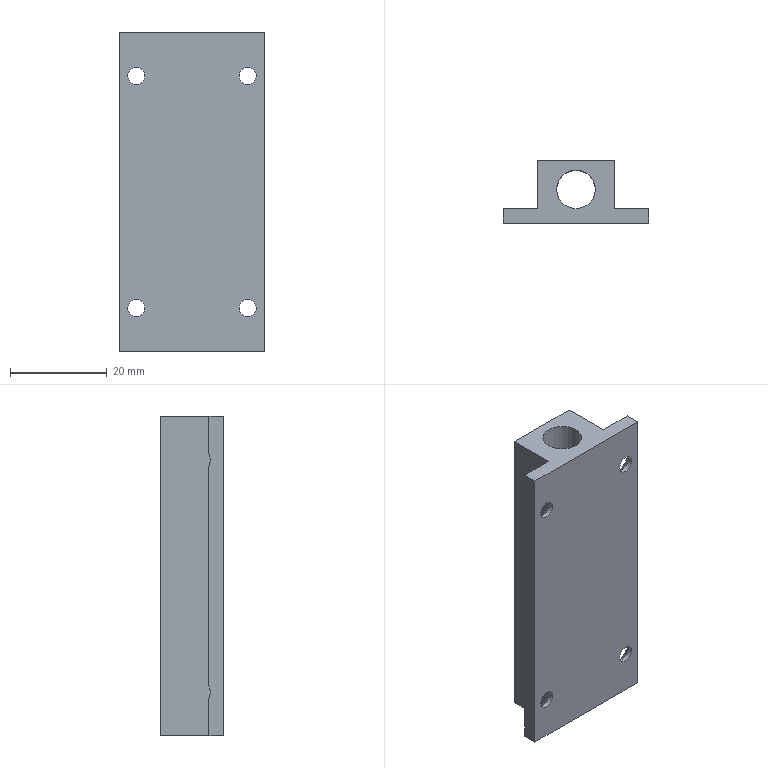Part | STEP file | latch | 1 solid | 23 faces | box 30 x 13 x 66 mm | volume 12946 mm3 | plane 14 | cylinder 5 | cone 4 | commonest cylinder face diameters 3.5 x4 8 x1